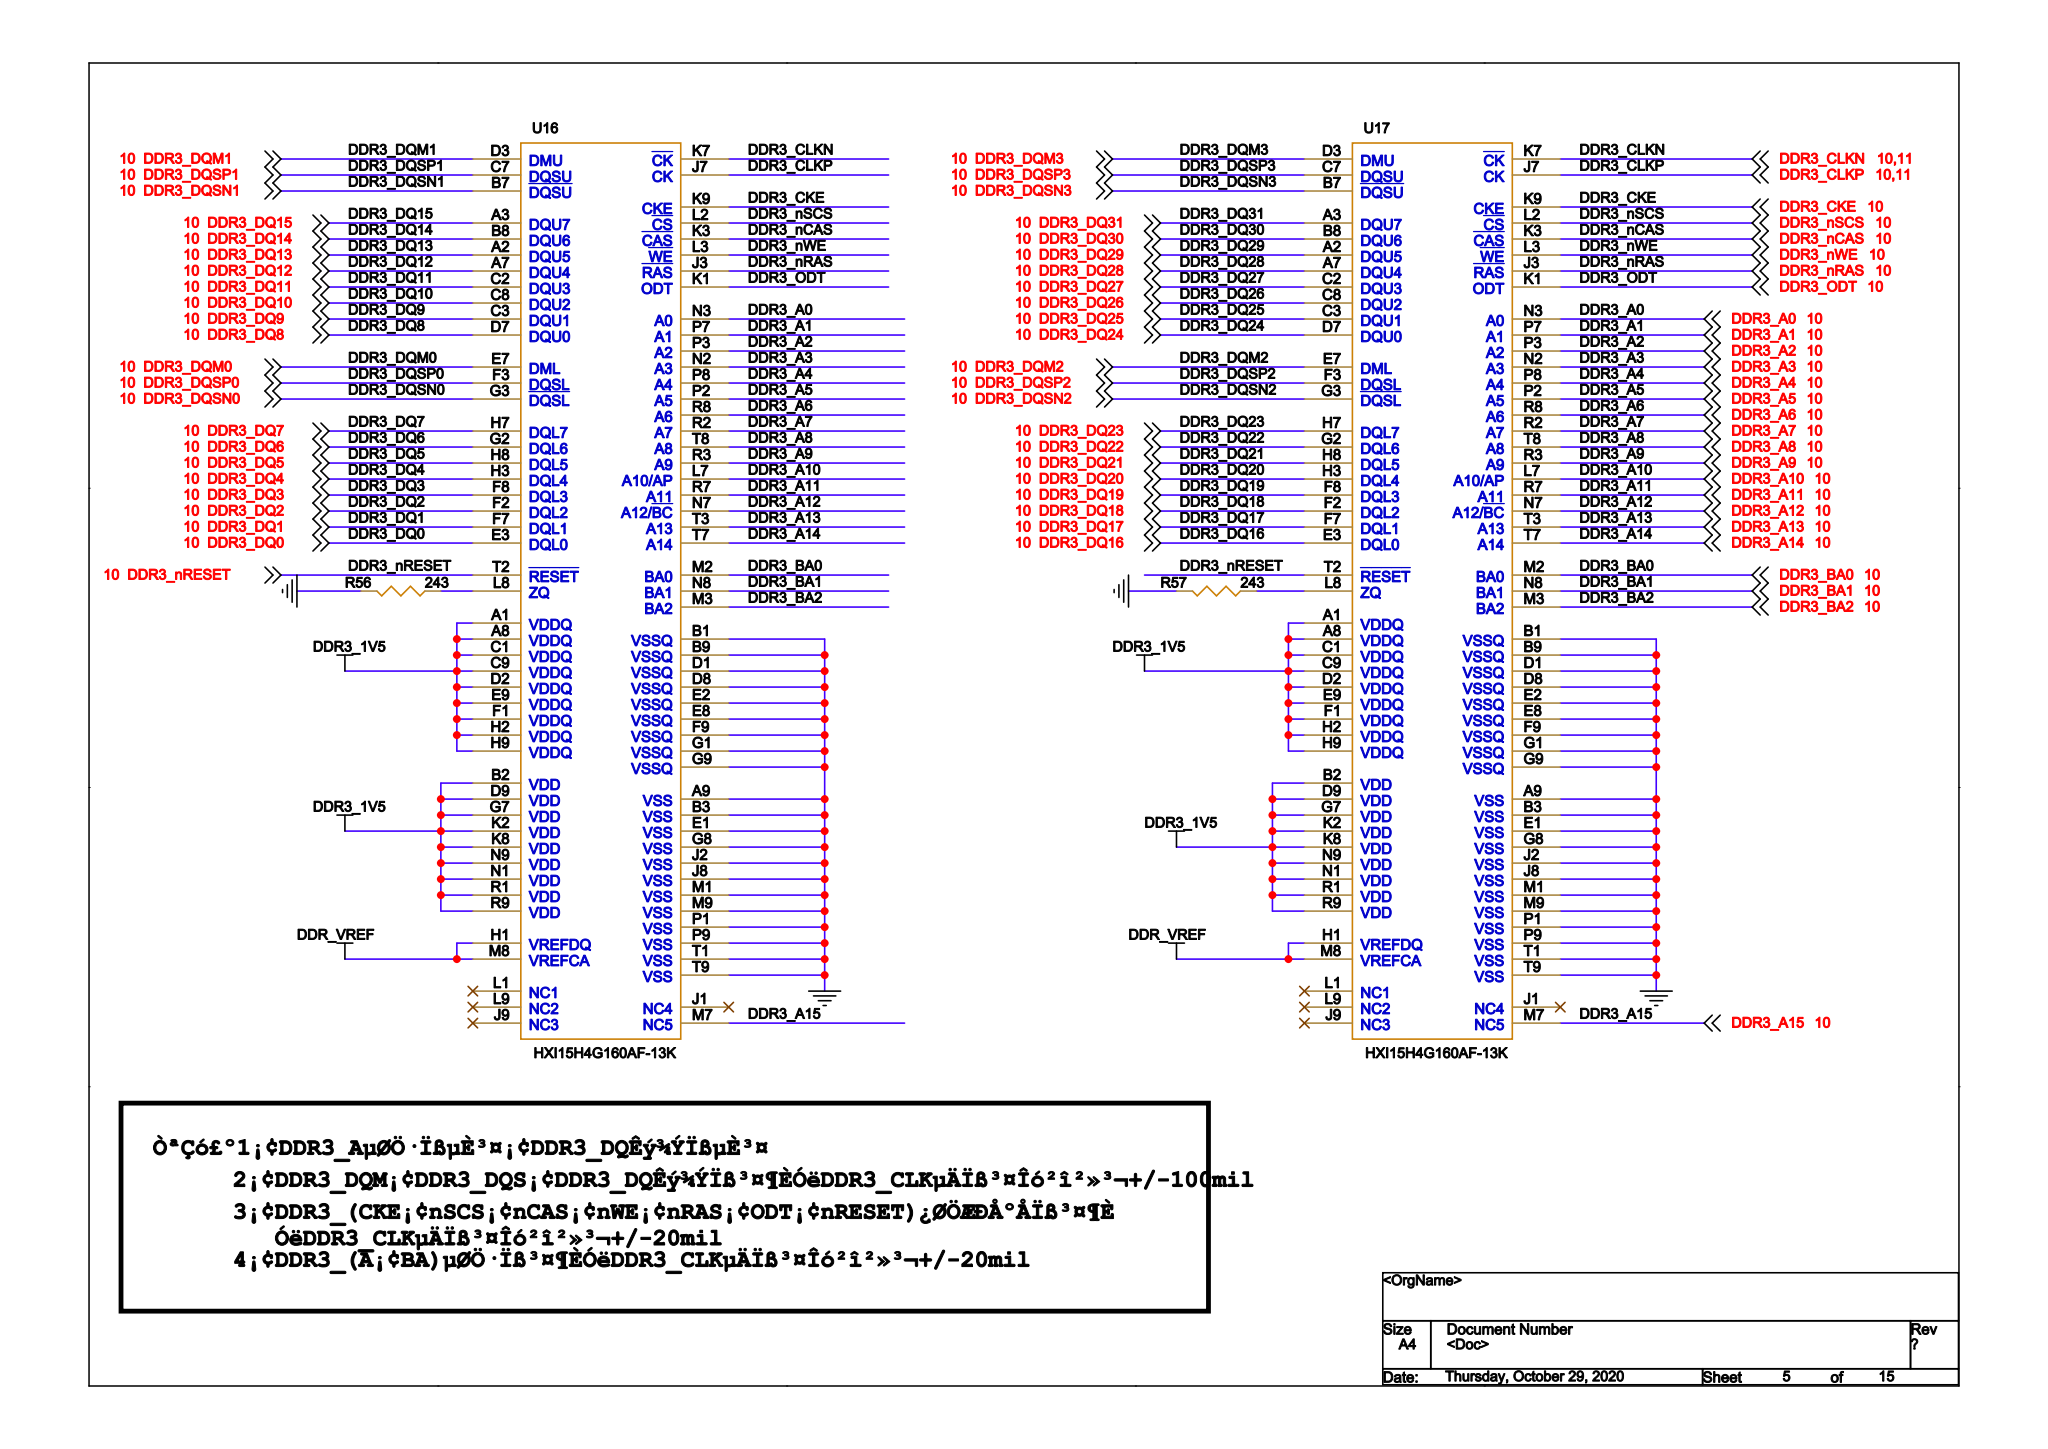Circuit board | Cadence Allegro | 406 parts | 392 nets | one sheet of the schematic
Parts on this sheet (reference | value | footprint):
R56 | 243 | R_0603
R57 | 243 | R_0603
U16 | HXI15H4G160AF-13K | U_TFBGA96
U17 | HXI15H4G160AF-13K | U_TFBGA96
Nets of these parts (net: part-pin ...):
GND: R56-2 R57-2 U16-A9 U16-B1 U16-B3 U16-B9 U16-D1 U16-D8 U16-E1 U16-E2 U16-E8 U16-F9 U16-G1 U16-G8 U16-G9 U16-J2 U16-J8 U16-M1 U16-M9 U16-P1 U16-P9 U16-T1 U16-T9 U17-A9 U17-B1 U17-B3 U17-B9 U17-D1 U17-D8 U17-E1 U17-E2 U17-E8 U17-F9 U17-G1 U17-G8 U17-G9 U17-J2 U17-J8 U17-M1 U17-M9 U17-P1 U17-P9 U17-T1 U17-T9
DDR3_1V5: U16-A1 U16-A8 U16-B2 U16-C1 U16-C9 U16-D2 U16-D9 U16-E9 U16-F1 U16-G7 U16-H2 U16-H9 U16-K2 U16-K8 U16-N1 U16-N9 U16-R1 U16-R9 U17-A1 U17-A8 U17-B2 U17-C1 U17-C9 U17-D2 U17-D9 U17-E9 U17-F1 U17-G7 U17-H2 U17-H9 U17-K2 U17-K8 U17-N1 U17-N9 U17-R1 U17-R9
DDR_VREF: U16-H1 U16-M8 U17-H1 U17-M8
DDR3_CLKN: U16-K7 U17-K7
DDR3_CLKP: U16-J7 U17-J7
DDR3_CKE: U16-K9 U17-K9
N16543936: R56-1 U16-L8
N16544626: R57-1 U17-L8
DDR3_BA1: U16-N8 U17-N8
DDR3_A15: U16-M7 U17-M7
DDR3_BA0: U16-M2 U17-M2
DDR3_A10: U16-L7 U17-L7
DDR3_ODT: U16-K1 U17-K1
DDR3_A8: U16-T8 U17-T8
DDR3_A13: U16-T3 U17-T3
DDR3_A12: U16-N7 U17-N7
DDR3_A1: U16-P7 U17-P7
DDR3_A4: U16-P8 U17-P8
DDR3_A6: U16-R8 U17-R8
DDR3_A14: U16-T7 U17-T7
DDR3_A11: U16-R7 U17-R7
DDR3_A5: U16-P2 U17-P2
DDR3_A2: U16-P3 U17-P3
DDR3_A7: U16-R2 U17-R2
DDR3_A9: U16-R3 U17-R3
DDR3_BA2: U16-M3 U17-M3
DDR3_A3: U16-N2 U17-N2
DDR3_A0: U16-N3 U17-N3
DDR3_DQM0: U16-E7
DDR3_DQM1: U16-D3
DDR3_DQ0: U16-E3
DDR3_DQ1: U16-F7
DDR3_DQ2: U16-F2
DDR3_DQ3: U16-F8
DDR3_DQ4: U16-H3
DDR3_DQ5: U16-H8
DDR3_DQ6: U16-G2
DDR3_DQ7: U16-H7
DDR3_DQSP0: U16-F3
DDR3_DQSP1: U16-C7
DDR3_DQ8: U16-D7
DDR3_DQ9: U16-C3
DDR3_DQ10: U16-C8
DDR3_DQ11: U16-C2
DDR3_DQ12: U16-A7
DDR3_DQ13: U16-A2
DDR3_DQ14: U16-B8
DDR3_DQ15: U16-A3
DDR3_DQSN0: U16-G3
DDR3_DQSN1: U16-B7
DDR3_DQM2: U17-E7
DDR3_DQM3: U17-D3
DDR3_DQ16: U17-E3
DDR3_DQ17: U17-F7
DDR3_DQ18: U17-F2
DDR3_DQ19: U17-F8
DDR3_DQ20: U17-H3
DDR3_DQ21: U17-H8
DDR3_DQ22: U17-G2
DDR3_DQ23: U17-H7
DDR3_DQSP2: U17-F3
DDR3_DQSP3: U17-C7
DDR3_DQ24: U17-D7
DDR3_DQ25: U17-C3
DDR3_DQ26: U17-C8
DDR3_DQ27: U17-C2
DDR3_DQ28: U17-A7
DDR3_DQ29: U17-A2
DDR3_DQ30: U17-B8
DDR3_DQ31: U17-A3
DDR3_DQSN2: U17-G3
DDR3_DQSN3: U17-B7